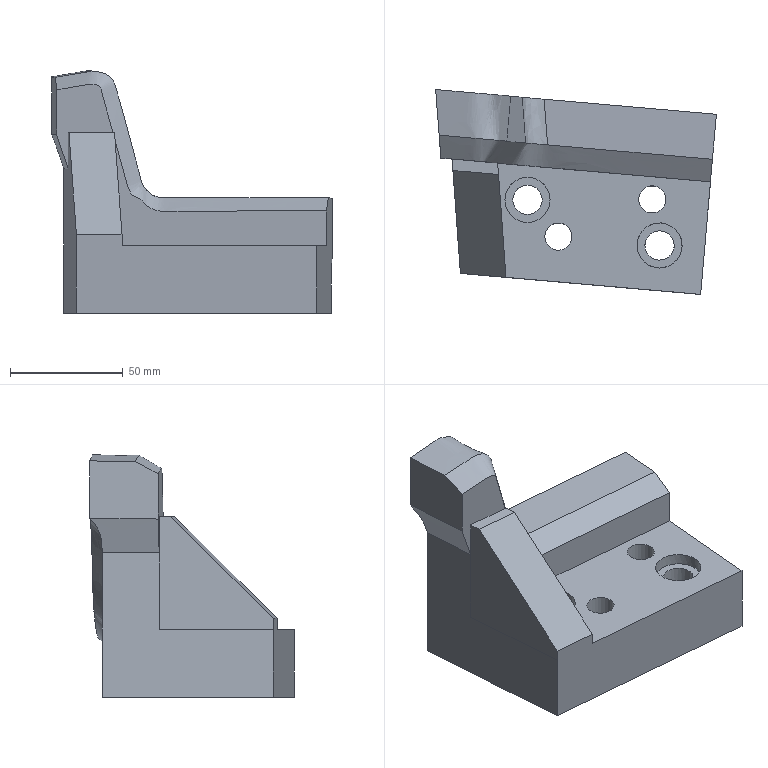Part | NX | features solid 2 | 1 solid | 29 faces | box 124.296 x 90.57 x 107.416 mm | volume 390261 mm3 | spline 13 | plane 10 | cylinder 6 | commonest cylinder face diameters 12 x2 13 x2 20 x2